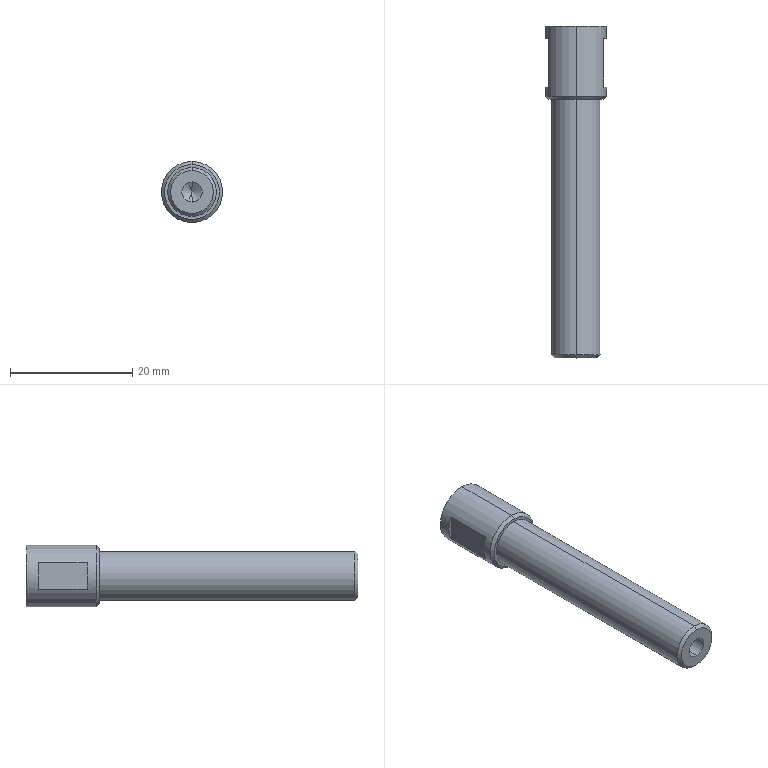Part | SolidWorks | features 3DProfileFeature 2, HoleWzd 2, ICE 2, Chamfer 1, Extrusion 1 | 1 solid | 25 faces | box 10 x 54.3 x 10 mm | volume 2772 mm3 | plane 9 | cone 8 | cylinder 8 | commonest cylinder face diameters 3.3 x2 4.2 x2 8 x2 10 x2
STEP:
#1=CARTESIAN_POINT('',(0.,0.,-3.5));
#2=VERTEX_POINT('',#1);
#3=CARTESIAN_POINT('',(0.,0.,3.5));
#4=VERTEX_POINT('',#3);
#5=CARTESIAN_POINT('',(0.,0.,0.));
#6=DIRECTION('',(0.,-1.,0.));
#7=DIRECTION('',(0.,0.,1.));
#8=AXIS2_PLACEMENT_3D('',#5,#6,#7);
#9=CIRCLE('',#8,3.5);
#10=EDGE_CURVE('',#2,#4,#9,.T.);
#11=ORIENTED_EDGE('',*,*,#10,.F.);
#12=CARTESIAN_POINT('',(0.,0.5,-4.));
#13=VERTEX_POINT('',#12);
#14=CARTESIAN_POINT('',(0.,0.5,-4.));
#15=DIRECTION('',(0.,0.7071,-0.7071));
#16=VECTOR('',#15,1000.);
#17=LINE('',#14,#16);
#18=EDGE_CURVE('',#2,#13,#17,.T.);
#19=ORIENTED_EDGE('',*,*,#18,.T.);
#20=CARTESIAN_POINT('',(0.,0.5,4.));
#21=VERTEX_POINT('',#20);
#22=CARTESIAN_POINT('',(0.,0.5,0.));
#23=DIRECTION('',(0.,1.,0.));
#24=DIRECTION('',(0.,0.,1.));
#25=AXIS2_PLACEMENT_3D('',#22,#23,#24);
#26=CIRCLE('',#25,4.);
#27=EDGE_CURVE('',#21,#13,#26,.T.);
#28=ORIENTED_EDGE('',*,*,#27,.F.);
#29=CARTESIAN_POINT('',(0.,0.5,4.));
#30=DIRECTION('',(0.,0.7071,0.7071));
#31=VECTOR('',#30,1000.);
#32=LINE('',#29,#31);
#33=EDGE_CURVE('',#4,#21,#32,.T.);
#34=ORIENTED_EDGE('',*,*,#33,.F.);
#35=EDGE_LOOP('',(#11,#19,#28,#34));
#36=FACE_OUTER_BOUND('',#35,.T.);
#37=CARTESIAN_POINT('',(0.,0.5,0.));
#38=DIRECTION('',(0.,1.,0.));
#39=DIRECTION('',(0.,0.,1.));
#40=AXIS2_PLACEMENT_3D('',#37,#38,#39);
#41=CONICAL_SURFACE('',#40,4.,0.7854);
#42=ADVANCED_FACE('',(#36),#41,.T.);
#43=CARTESIAN_POINT('',(0.,42.3,-4.5));
#44=VERTEX_POINT('',#43);
#45=CARTESIAN_POINT('',(0.,42.3,4.5));
#46=VERTEX_POINT('',#45);
#47=CARTESIAN_POINT('',(0.,42.3,0.));
#48=DIRECTION('',(0.,-1.,0.));
#49=DIRECTION('',(0.,0.,1.));
#50=AXIS2_PLACEMENT_3D('',#47,#48,#49);
#51=CIRCLE('',#50,4.5);
#52=EDGE_CURVE('',#44,#46,#51,.T.);
#53=ORIENTED_EDGE('',*,*,#52,.F.);
#54=CARTESIAN_POINT('',(0.,42.8,-5.));
#55=VERTEX_POINT('',#54);
#56=CARTESIAN_POINT('',(0.,42.8,-5.));
#57=DIRECTION('',(0.,0.7071,-0.7071));
#58=VECTOR('',#57,1000.);
#59=LINE('',#56,#58);
#60=EDGE_CURVE('',#44,#55,#59,.T.);
#61=ORIENTED_EDGE('',*,*,#60,.T.);
#62=CARTESIAN_POINT('',(0.,42.8,5.));
#63=VERTEX_POINT('',#62);
#64=CARTESIAN_POINT('',(0.,42.8,0.));
#65=DIRECTION('',(0.,1.,0.));
#66=DIRECTION('',(0.,0.,1.));
#67=AXIS2_PLACEMENT_3D('',#64,#65,#66);
#68=CIRCLE('',#67,5.);
#69=EDGE_CURVE('',#63,#55,#68,.T.);
#70=ORIENTED_EDGE('',*,*,#69,.F.);
#71=CARTESIAN_POINT('',(0.,42.8,5.));
#72=DIRECTION('',(0.,0.7071,0.7071));
#73=VECTOR('',#72,1000.);
#74=LINE('',#71,#73);
#75=EDGE_CURVE('',#46,#63,#74,.T.);
#76=ORIENTED_EDGE('',*,*,#75,.F.);
#77=EDGE_LOOP('',(#53,#61,#70,#76));
#78=FACE_OUTER_BOUND('',#77,.T.);
#79=CARTESIAN_POINT('',(0.,42.8,0.));
#80=DIRECTION('',(0.,1.,0.));
#81=DIRECTION('',(0.,0.,1.));
#82=AXIS2_PLACEMENT_3D('',#79,#80,#81);
#83=CONICAL_SURFACE('',#82,5.,0.7854);
#84=ADVANCED_FACE('',(#78),#83,.T.);
#85=CARTESIAN_POINT('',(0.,10.1,1.65));
#86=VERTEX_POINT('',#85);
#87=CARTESIAN_POINT('',(0.,10.1,-1.65));
#88=VERTEX_POINT('',#87);
#89=CARTESIAN_POINT('',(0.,10.1,0.));
#90=DIRECTION('',(0.,-1.,0.));
#91=DIRECTION('',(0.,0.,-1.));
#92=AXIS2_PLACEMENT_3D('',#89,#90,#91);
#93=CIRCLE('',#92,1.65);
#94=EDGE_CURVE('',#86,#88,#93,.T.);
#95=ORIENTED_EDGE('',*,*,#94,.F.);
#96=CARTESIAN_POINT('',(0.,0.,1.65));
#97=VERTEX_POINT('',#96);
#98=CARTESIAN_POINT('',(0.,0.,1.65));
#99=DIRECTION('',(0.,-1.,0.));
#100=VECTOR('',#99,1000.);
#101=LINE('',#98,#100);
#102=EDGE_CURVE('',#86,#97,#101,.T.);
#103=ORIENTED_EDGE('',*,*,#102,.T.);
#104=CARTESIAN_POINT('',(0.,0.,-1.65));
#105=VERTEX_POINT('',#104);
#106=CARTESIAN_POINT('',(0.,0.,0.));
#107=DIRECTION('',(0.,-1.,0.));
#108=DIRECTION('',(0.,0.,-1.));
#109=AXIS2_PLACEMENT_3D('',#106,#107,#108);
#110=CIRCLE('',#109,1.65);
#111=EDGE_CURVE('',#97,#105,#110,.T.);
#112=ORIENTED_EDGE('',*,*,#111,.T.);
#113=CARTESIAN_POINT('',(0.,0.,-1.65));
#114=DIRECTION('',(0.,-1.,0.));
#115=VECTOR('',#114,1000.);
#116=LINE('',#113,#115);
#117=EDGE_CURVE('',#88,#105,#116,.T.);
#118=ORIENTED_EDGE('',*,*,#117,.F.);
#119=EDGE_LOOP('',(#95,#103,#112,#118));
#120=FACE_OUTER_BOUND('',#119,.T.);
#121=CARTESIAN_POINT('',(0.,0.,0.));
#122=DIRECTION('',(0.,-1.,0.));
#123=DIRECTION('',(0.,0.,-1.));
#124=AXIS2_PLACEMENT_3D('',#121,#122,#123);
#125=CYLINDRICAL_SURFACE('',#124,1.65);
#126=ADVANCED_FACE('',(#120),#125,.F.);
#127=CARTESIAN_POINT('',(0.,11.091,0.));
#128=VERTEX_POINT('',#127);
#129=CARTESIAN_POINT('',(0.,10.1,-1.65));
#130=DIRECTION('',(0.,-0.515,-0.8572));
#131=VECTOR('',#130,1000.);
#132=LINE('',#129,#131);
#133=EDGE_CURVE('',#128,#88,#132,.T.);
#134=ORIENTED_EDGE('',*,*,#133,.F.);
#135=CARTESIAN_POINT('',(0.,10.1,1.65));
#136=DIRECTION('',(0.,-0.515,0.8572));
#137=VECTOR('',#136,1000.);
#138=LINE('',#135,#137);
#139=EDGE_CURVE('',#128,#86,#138,.T.);
#140=ORIENTED_EDGE('',*,*,#139,.T.);
#141=ORIENTED_EDGE('',*,*,#94,.T.);
#142=EDGE_LOOP('',(#134,#140,#141));
#143=FACE_OUTER_BOUND('',#142,.T.);
#144=CARTESIAN_POINT('',(0.,10.1,0.));
#145=DIRECTION('',(0.,-1.,0.));
#146=DIRECTION('',(0.,0.,-1.));
#147=AXIS2_PLACEMENT_3D('',#144,#145,#146);
#148=CONICAL_SURFACE('',#147,1.65,1.03);
#149=ADVANCED_FACE('',(#143),#148,.F.);
#150=CARTESIAN_POINT('',(0.,41.9,-2.1));
#151=VERTEX_POINT('',#150);
#152=CARTESIAN_POINT('',(0.,41.9,2.1));
#153=VERTEX_POINT('',#152);
#154=CARTESIAN_POINT('',(0.,41.9,0.));
#155=DIRECTION('',(0.,1.,0.));
#156=DIRECTION('',(0.,0.,1.));
#157=AXIS2_PLACEMENT_3D('',#154,#155,#156);
#158=CIRCLE('',#157,2.1);
#159=EDGE_CURVE('',#151,#153,#158,.T.);
#160=ORIENTED_EDGE('',*,*,#159,.F.);
#161=CARTESIAN_POINT('',(0.,54.3,-2.1));
#162=VERTEX_POINT('',#161);
#163=CARTESIAN_POINT('',(0.,54.3,-2.1));
#164=DIRECTION('',(0.,1.,0.));
#165=VECTOR('',#164,1000.);
#166=LINE('',#163,#165);
#167=EDGE_CURVE('',#151,#162,#166,.T.);
#168=ORIENTED_EDGE('',*,*,#167,.T.);
#169=CARTESIAN_POINT('',(0.,54.3,2.1));
#170=VERTEX_POINT('',#169);
#171=CARTESIAN_POINT('',(0.,54.3,0.));
#172=DIRECTION('',(0.,1.,0.));
#173=DIRECTION('',(0.,0.,1.));
#174=AXIS2_PLACEMENT_3D('',#171,#172,#173);
#175=CIRCLE('',#174,2.1);
#176=EDGE_CURVE('',#162,#170,#175,.T.);
#177=ORIENTED_EDGE('',*,*,#176,.T.);
#178=CARTESIAN_POINT('',(0.,54.3,2.1));
#179=DIRECTION('',(0.,1.,0.));
#180=VECTOR('',#179,1000.);
#181=LINE('',#178,#180);
#182=EDGE_CURVE('',#153,#170,#181,.T.);
#183=ORIENTED_EDGE('',*,*,#182,.F.);
#184=EDGE_LOOP('',(#160,#168,#177,#183));
#185=FACE_OUTER_BOUND('',#184,.T.);
#186=CARTESIAN_POINT('',(0.,54.3,0.));
#187=DIRECTION('',(0.,1.,0.));
#188=DIRECTION('',(0.,0.,1.));
#189=AXIS2_PLACEMENT_3D('',#186,#187,#188);
#190=CYLINDRICAL_SURFACE('',#189,2.1);
#191=ADVANCED_FACE('',(#185),#190,.F.);
#192=CARTESIAN_POINT('',(0.,40.638,0.));
#193=VERTEX_POINT('',#192);
#194=CARTESIAN_POINT('',(0.,41.9,2.1));
#195=DIRECTION('',(0.,0.515,0.8572));
#196=VECTOR('',#195,1000.);
#197=LINE('',#194,#196);
#198=EDGE_CURVE('',#193,#153,#197,.T.);
#199=ORIENTED_EDGE('',*,*,#198,.F.);
#200=CARTESIAN_POINT('',(0.,41.9,-2.1));
#201=DIRECTION('',(0.,0.515,-0.8572));
#202=VECTOR('',#201,1000.);
#203=LINE('',#200,#202);
#204=EDGE_CURVE('',#193,#151,#203,.T.);
#205=ORIENTED_EDGE('',*,*,#204,.T.);
#206=ORIENTED_EDGE('',*,*,#159,.T.);
#207=EDGE_LOOP('',(#199,#205,#206));
#208=FACE_OUTER_BOUND('',#207,.T.);
#209=CARTESIAN_POINT('',(0.,41.9,0.));
#210=DIRECTION('',(0.,1.,0.));
#211=DIRECTION('',(0.,0.,1.));
#212=AXIS2_PLACEMENT_3D('',#209,#210,#211);
#213=CONICAL_SURFACE('',#212,2.1,1.03);
#214=ADVANCED_FACE('',(#208),#213,.F.);
#215=CARTESIAN_POINT('',(4.5,52.3,-2.179));
#216=VERTEX_POINT('',#215);
#217=CARTESIAN_POINT('',(4.5,44.3,-2.179));
#218=VERTEX_POINT('',#217);
#219=CARTESIAN_POINT('',(4.5,54.3,-2.179));
#220=DIRECTION('',(0.,-1.,0.));
#221=VECTOR('',#220,1000.);
#222=LINE('',#219,#221);
#223=EDGE_CURVE('',#216,#218,#222,.T.);
#224=ORIENTED_EDGE('',*,*,#223,.T.);
#225=CARTESIAN_POINT('',(4.5,44.3,2.179));
#226=VERTEX_POINT('',#225);
#227=CARTESIAN_POINT('',(0.,44.3,0.));
#228=DIRECTION('',(0.,-1.,0.));
#229=DIRECTION('',(0.,0.,-1.));
#230=AXIS2_PLACEMENT_3D('',#227,#228,#229);
#231=CIRCLE('',#230,5.);
#232=EDGE_CURVE('',#218,#226,#231,.T.);
#233=ORIENTED_EDGE('',*,*,#232,.T.);
#234=CARTESIAN_POINT('',(4.5,52.3,2.179));
#235=VERTEX_POINT('',#234);
#236=CARTESIAN_POINT('',(4.5,54.3,2.179));
#237=DIRECTION('',(0.,1.,0.));
#238=VECTOR('',#237,1000.);
#239=LINE('',#236,#238);
#240=EDGE_CURVE('',#226,#235,#239,.T.);
#241=ORIENTED_EDGE('',*,*,#240,.T.);
#242=CARTESIAN_POINT('',(0.,52.3,0.));
#243=DIRECTION('',(0.,1.,0.));
#244=DIRECTION('',(0.,0.,1.));
#245=AXIS2_PLACEMENT_3D('',#242,#243,#244);
#246=CIRCLE('',#245,5.);
#247=EDGE_CURVE('',#235,#216,#246,.T.);
#248=ORIENTED_EDGE('',*,*,#247,.T.);
#249=EDGE_LOOP('',(#224,#233,#241,#248));
#250=FACE_BOUND('',#249,.T.);
#251=CARTESIAN_POINT('',(0.,54.3,5.));
#252=VERTEX_POINT('',#251);
#253=CARTESIAN_POINT('',(0.,54.3,-5.));
#254=VERTEX_POINT('',#253);
#255=CARTESIAN_POINT('',(0.,54.3,0.));
#256=DIRECTION('',(0.,1.,0.));
#257=DIRECTION('',(0.,0.,1.));
#258=AXIS2_PLACEMENT_3D('',#255,#256,#257);
#259=CIRCLE('',#258,5.);
#260=EDGE_CURVE('',#252,#254,#259,.T.);
#261=ORIENTED_EDGE('',*,*,#260,.F.);
#262=CARTESIAN_POINT('',(0.,54.3,5.));
#263=DIRECTION('',(0.,-1.,0.));
#264=VECTOR('',#263,1000.);
#265=LINE('',#262,#264);
#266=EDGE_CURVE('',#252,#63,#265,.T.);
#267=ORIENTED_EDGE('',*,*,#266,.T.);
#268=ORIENTED_EDGE('',*,*,#69,.T.);
#269=CARTESIAN_POINT('',(0.,54.3,-5.));
#270=DIRECTION('',(0.,-1.,0.));
#271=VECTOR('',#270,1000.);
#272=LINE('',#269,#271);
#273=EDGE_CURVE('',#254,#55,#272,.T.);
#274=ORIENTED_EDGE('',*,*,#273,.F.);
#275=EDGE_LOOP('',(#261,#267,#268,#274));
#276=FACE_OUTER_BOUND('',#275,.T.);
#277=CARTESIAN_POINT('',(0.,54.3,0.));
#278=DIRECTION('',(0.,-1.,0.));
#279=DIRECTION('',(0.,0.,-1.));
#280=AXIS2_PLACEMENT_3D('',#277,#278,#279);
#281=CYLINDRICAL_SURFACE('',#280,5.);
#282=ADVANCED_FACE('',(#250,#276),#281,.T.);
#283=CARTESIAN_POINT('',(0.,42.3,4.));
#284=VERTEX_POINT('',#283);
#285=CARTESIAN_POINT('',(0.,42.3,-4.));
#286=VERTEX_POINT('',#285);
#287=CARTESIAN_POINT('',(0.,42.3,0.));
#288=DIRECTION('',(0.,1.,0.));
#289=DIRECTION('',(0.,0.,1.));
#290=AXIS2_PLACEMENT_3D('',#287,#288,#289);
#291=CIRCLE('',#290,4.);
#292=EDGE_CURVE('',#284,#286,#291,.T.);
#293=ORIENTED_EDGE('',*,*,#292,.F.);
#294=CARTESIAN_POINT('',(0.,42.3,4.));
#295=DIRECTION('',(0.,-1.,0.));
#296=VECTOR('',#295,1000.);
#297=LINE('',#294,#296);
#298=EDGE_CURVE('',#284,#21,#297,.T.);
#299=ORIENTED_EDGE('',*,*,#298,.T.);
#300=ORIENTED_EDGE('',*,*,#27,.T.);
#301=CARTESIAN_POINT('',(0.,42.3,-4.));
#302=DIRECTION('',(0.,-1.,0.));
#303=VECTOR('',#302,1000.);
#304=LINE('',#301,#303);
#305=EDGE_CURVE('',#286,#13,#304,.T.);
#306=ORIENTED_EDGE('',*,*,#305,.F.);
#307=EDGE_LOOP('',(#293,#299,#300,#306));
#308=FACE_OUTER_BOUND('',#307,.T.);
#309=CARTESIAN_POINT('',(0.,42.3,0.));
#310=DIRECTION('',(0.,-1.,0.));
#311=DIRECTION('',(0.,0.,-1.));
#312=AXIS2_PLACEMENT_3D('',#309,#310,#311);
#313=CYLINDRICAL_SURFACE('',#312,4.);
#314=ADVANCED_FACE('',(#308),#313,.T.);
#315=ORIENTED_EDGE('',*,*,#298,.F.);
#316=CARTESIAN_POINT('',(0.,42.3,0.));
#317=DIRECTION('',(0.,1.,0.));
#318=DIRECTION('',(0.,0.,1.));
#319=AXIS2_PLACEMENT_3D('',#316,#317,#318);
#320=CIRCLE('',#319,4.);
#321=EDGE_CURVE('',#286,#284,#320,.T.);
#322=ORIENTED_EDGE('',*,*,#321,.F.);
#323=ORIENTED_EDGE('',*,*,#305,.T.);
#324=CARTESIAN_POINT('',(0.,0.5,0.));
#325=DIRECTION('',(0.,1.,0.));
#326=DIRECTION('',(0.,0.,1.));
#327=AXIS2_PLACEMENT_3D('',#324,#325,#326);
#328=CIRCLE('',#327,4.);
#329=EDGE_CURVE('',#13,#21,#328,.T.);
#330=ORIENTED_EDGE('',*,*,#329,.T.);
#331=EDGE_LOOP('',(#315,#322,#323,#330));
#332=FACE_OUTER_BOUND('',#331,.T.);
#333=CARTESIAN_POINT('',(0.,42.3,0.));
#334=DIRECTION('',(0.,-1.,0.));
#335=DIRECTION('',(0.,0.,-1.));
#336=AXIS2_PLACEMENT_3D('',#333,#334,#335);
#337=CYLINDRICAL_SURFACE('',#336,4.);
#338=ADVANCED_FACE('',(#332),#337,.T.);
#339=CARTESIAN_POINT('',(0.,0.,0.));
#340=DIRECTION('',(0.,-1.,0.));
#341=DIRECTION('',(0.,0.,1.));
#342=AXIS2_PLACEMENT_3D('',#339,#340,#341);
#343=CIRCLE('',#342,3.5);
#344=EDGE_CURVE('',#4,#2,#343,.T.);
#345=ORIENTED_EDGE('',*,*,#344,.T.);
#346=ORIENTED_EDGE('',*,*,#10,.T.);
#347=EDGE_LOOP('',(#345,#346));
#348=FACE_OUTER_BOUND('',#347,.T.);
#349=CARTESIAN_POINT('',(0.,0.,0.));
#350=DIRECTION('',(0.,-1.,0.));
#351=DIRECTION('',(0.,0.,-1.));
#352=AXIS2_PLACEMENT_3D('',#349,#350,#351);
#353=CIRCLE('',#352,1.65);
#354=EDGE_CURVE('',#105,#97,#353,.T.);
#355=ORIENTED_EDGE('',*,*,#354,.F.);
#356=ORIENTED_EDGE('',*,*,#111,.F.);
#357=EDGE_LOOP('',(#355,#356));
#358=FACE_BOUND('',#357,.T.);
#359=CARTESIAN_POINT('',(0.,0.,0.));
#360=DIRECTION('',(0.,1.,0.));
#361=DIRECTION('',(0.,0.,1.));
#362=AXIS2_PLACEMENT_3D('',#359,#360,#361);
#363=PLANE('',#362);
#364=ADVANCED_FACE('',(#348,#358),#363,.F.);
#365=CARTESIAN_POINT('',(0.,42.3,0.));
#366=DIRECTION('',(0.,-1.,0.));
#367=DIRECTION('',(0.,0.,1.));
#368=AXIS2_PLACEMENT_3D('',#365,#366,#367);
#369=CIRCLE('',#368,4.5);
#370=EDGE_CURVE('',#46,#44,#369,.T.);
#371=ORIENTED_EDGE('',*,*,#370,.T.);
#372=ORIENTED_EDGE('',*,*,#52,.T.);
#373=EDGE_LOOP('',(#371,#372));
#374=FACE_OUTER_BOUND('',#373,.T.);
#375=ORIENTED_EDGE('',*,*,#321,.T.);
#376=ORIENTED_EDGE('',*,*,#292,.T.);
#377=EDGE_LOOP('',(#375,#376));
#378=FACE_BOUND('',#377,.T.);
#379=CARTESIAN_POINT('',(0.,42.3,0.));
#380=DIRECTION('',(0.,1.,0.));
#381=DIRECTION('',(0.,0.,1.));
#382=AXIS2_PLACEMENT_3D('',#379,#380,#381);
#383=PLANE('',#382);
#384=ADVANCED_FACE('',(#374,#378),#383,.F.);
#385=ORIENTED_EDGE('',*,*,#266,.F.);
#386=CARTESIAN_POINT('',(0.,54.3,0.));
#387=DIRECTION('',(0.,1.,0.));
#388=DIRECTION('',(0.,0.,1.));
#389=AXIS2_PLACEMENT_3D('',#386,#387,#388);
#390=CIRCLE('',#389,5.);
#391=EDGE_CURVE('',#254,#252,#390,.T.);
#392=ORIENTED_EDGE('',*,*,#391,.F.);
#393=ORIENTED_EDGE('',*,*,#273,.T.);
#394=CARTESIAN_POINT('',(0.,42.8,0.));
#395=DIRECTION('',(0.,1.,0.));
#396=DIRECTION('',(0.,0.,1.));
#397=AXIS2_PLACEMENT_3D('',#394,#395,#396);
#398=CIRCLE('',#397,5.);
#399=EDGE_CURVE('',#55,#63,#398,.T.);
#400=ORIENTED_EDGE('',*,*,#399,.T.);
#401=EDGE_LOOP('',(#385,#392,#393,#400));
#402=FACE_OUTER_BOUND('',#401,.T.);
#403=CARTESIAN_POINT('',(-4.5,52.3,2.179));
#404=VERTEX_POINT('',#403);
#405=CARTESIAN_POINT('',(-4.5,44.3,2.179));
#406=VERTEX_POINT('',#405);
#407=CARTESIAN_POINT('',(-4.5,54.3,2.179));
#408=DIRECTION('',(0.,-1.,0.));
#409=VECTOR('',#408,1000.);
#410=LINE('',#407,#409);
#411=EDGE_CURVE('',#404,#406,#410,.T.);
#412=ORIENTED_EDGE('',*,*,#411,.T.);
#413=CARTESIAN_POINT('',(-4.5,44.3,-2.179));
#414=VERTEX_POINT('',#413);
#415=CARTESIAN_POINT('',(0.,44.3,0.));
#416=DIRECTION('',(0.,-1.,0.));
#417=DIRECTION('',(0.,0.,-1.));
#418=AXIS2_PLACEMENT_3D('',#415,#416,#417);
#419=CIRCLE('',#418,5.);
#420=EDGE_CURVE('',#406,#414,#419,.T.);
#421=ORIENTED_EDGE('',*,*,#420,.T.);
#422=CARTESIAN_POINT('',(-4.5,52.3,-2.179));
#423=VERTEX_POINT('',#422);
#424=CARTESIAN_POINT('',(-4.5,54.3,-2.179));
#425=DIRECTION('',(0.,1.,0.));
#426=VECTOR('',#425,1000.);
#427=LINE('',#424,#426);
#428=EDGE_CURVE('',#414,#423,#427,.T.);
#429=ORIENTED_EDGE('',*,*,#428,.T.);
#430=CARTESIAN_POINT('',(0.,52.3,0.));
#431=DIRECTION('',(0.,1.,0.));
#432=DIRECTION('',(0.,0.,1.));
#433=AXIS2_PLACEMENT_3D('',#430,#431,#432);
#434=CIRCLE('',#433,5.);
#435=EDGE_CURVE('',#423,#404,#434,.T.);
#436=ORIENTED_EDGE('',*,*,#435,.T.);
#437=EDGE_LOOP('',(#412,#421,#429,#436));
#438=FACE_BOUND('',#437,.T.);
#439=CARTESIAN_POINT('',(0.,54.3,0.));
#440=DIRECTION('',(0.,-1.,0.));
#441=DIRECTION('',(0.,0.,-1.));
#442=AXIS2_PLACEMENT_3D('',#439,#440,#441);
#443=CYLINDRICAL_SURFACE('',#442,5.);
#444=ADVANCED_FACE('',(#402,#438),#443,.T.);
#445=CARTESIAN_POINT('',(0.,54.3,0.));
#446=DIRECTION('',(0.,1.,0.));
#447=DIRECTION('',(0.,0.,1.));
#448=AXIS2_PLACEMENT_3D('',#445,#446,#447);
#449=CIRCLE('',#448,2.1);
#450=EDGE_CURVE('',#170,#162,#449,.T.);
#451=ORIENTED_EDGE('',*,*,#450,.F.);
#452=ORIENTED_EDGE('',*,*,#176,.F.);
#453=EDGE_LOOP('',(#451,#452));
#454=FACE_BOUND('',#453,.T.);
#455=ORIENTED_EDGE('',*,*,#391,.T.);
#456=ORIENTED_EDGE('',*,*,#260,.T.);
#457=EDGE_LOOP('',(#455,#456));
#458=FACE_OUTER_BOUND('',#457,.T.);
#459=CARTESIAN_POINT('',(0.,54.3,0.));
#460=DIRECTION('',(0.,1.,0.));
#461=DIRECTION('',(0.,0.,1.));
#462=AXIS2_PLACEMENT_3D('',#459,#460,#461);
#463=PLANE('',#462);
#464=ADVANCED_FACE('',(#454,#458),#463,.T.);
#465=ORIENTED_EDGE('',*,*,#204,.F.);
#466=ORIENTED_EDGE('',*,*,#198,.T.);
#467=CARTESIAN_POINT('',(0.,41.9,0.));
#468=DIRECTION('',(0.,1.,0.));
#469=DIRECTION('',(0.,0.,1.));
#470=AXIS2_PLACEMENT_3D('',#467,#468,#469);
#471=CIRCLE('',#470,2.1);
#472=EDGE_CURVE('',#153,#151,#471,.T.);
#473=ORIENTED_EDGE('',*,*,#472,.T.);
#474=EDGE_LOOP('',(#465,#466,#473));
#475=FACE_OUTER_BOUND('',#474,.T.);
#476=CARTESIAN_POINT('',(0.,41.9,0.));
#477=DIRECTION('',(0.,1.,0.));
#478=DIRECTION('',(0.,0.,1.));
#479=AXIS2_PLACEMENT_3D('',#476,#477,#478);
#480=CONICAL_SURFACE('',#479,2.1,1.03);
#481=ADVANCED_FACE('',(#475),#480,.F.);
#482=ORIENTED_EDGE('',*,*,#167,.F.);
#483=ORIENTED_EDGE('',*,*,#472,.F.);
#484=ORIENTED_EDGE('',*,*,#182,.T.);
#485=ORIENTED_EDGE('',*,*,#450,.T.);
#486=EDGE_LOOP('',(#482,#483,#484,#485));
#487=FACE_OUTER_BOUND('',#486,.T.);
#488=CARTESIAN_POINT('',(0.,54.3,0.));
#489=DIRECTION('',(0.,1.,0.));
#490=DIRECTION('',(0.,0.,1.));
#491=AXIS2_PLACEMENT_3D('',#488,#489,#490);
#492=CYLINDRICAL_SURFACE('',#491,2.1);
#493=ADVANCED_FACE('',(#487),#492,.F.);
#494=ORIENTED_EDGE('',*,*,#139,.F.);
#495=ORIENTED_EDGE('',*,*,#133,.T.);
#496=CARTESIAN_POINT('',(0.,10.1,0.));
#497=DIRECTION('',(0.,-1.,0.));
#498=DIRECTION('',(0.,0.,-1.));
#499=AXIS2_PLACEMENT_3D('',#496,#497,#498);
#500=CIRCLE('',#499,1.65);
#501=EDGE_CURVE('',#88,#86,#500,.T.);
#502=ORIENTED_EDGE('',*,*,#501,.T.);
#503=EDGE_LOOP('',(#494,#495,#502));
#504=FACE_OUTER_BOUND('',#503,.T.);
#505=CARTESIAN_POINT('',(0.,10.1,0.));
#506=DIRECTION('',(0.,-1.,0.));
#507=DIRECTION('',(0.,0.,-1.));
#508=AXIS2_PLACEMENT_3D('',#505,#506,#507);
#509=CONICAL_SURFACE('',#508,1.65,1.03);
#510=ADVANCED_FACE('',(#504),#509,.F.);
#511=ORIENTED_EDGE('',*,*,#102,.F.);
#512=ORIENTED_EDGE('',*,*,#501,.F.);
#513=ORIENTED_EDGE('',*,*,#117,.T.);
#514=ORIENTED_EDGE('',*,*,#354,.T.);
#515=EDGE_LOOP('',(#511,#512,#513,#514));
#516=FACE_OUTER_BOUND('',#515,.T.);
#517=CARTESIAN_POINT('',(0.,0.,0.));
#518=DIRECTION('',(0.,-1.,0.));
#519=DIRECTION('',(0.,0.,-1.));
#520=AXIS2_PLACEMENT_3D('',#517,#518,#519);
#521=CYLINDRICAL_SURFACE('',#520,1.65);
#522=ADVANCED_FACE('',(#516),#521,.F.);
#523=CARTESIAN_POINT('',(-4.5,52.3,-5.));
#524=DIRECTION('',(0.,0.,1.));
#525=VECTOR('',#524,1000.);
#526=LINE('',#523,#525);
#527=EDGE_CURVE('',#423,#404,#526,.T.);
#528=ORIENTED_EDGE('',*,*,#527,.F.);
#529=ORIENTED_EDGE('',*,*,#428,.F.);
#530=CARTESIAN_POINT('',(-4.5,44.3,-5.));
#531=DIRECTION('',(0.,0.,1.));
#532=VECTOR('',#531,1000.);
#533=LINE('',#530,#532);
#534=EDGE_CURVE('',#414,#406,#533,.T.);
#535=ORIENTED_EDGE('',*,*,#534,.T.);
#536=ORIENTED_EDGE('',*,*,#411,.F.);
#537=EDGE_LOOP('',(#528,#529,#535,#536));
#538=FACE_OUTER_BOUND('',#537,.T.);
#539=CARTESIAN_POINT('',(-4.5,52.3,-5.));
#540=DIRECTION('',(1.,0.,0.));
#541=DIRECTION('',(0.,0.,-1.));
#542=AXIS2_PLACEMENT_3D('',#539,#540,#541);
#543=PLANE('',#542);
#544=ADVANCED_FACE('',(#538),#543,.F.);
#545=ORIENTED_EDGE('',*,*,#534,.F.);
#546=ORIENTED_EDGE('',*,*,#420,.F.);
#547=EDGE_LOOP('',(#545,#546));
#548=FACE_OUTER_BOUND('',#547,.T.);
#549=CARTESIAN_POINT('',(-5.5,44.3,-5.));
#550=DIRECTION('',(0.,-1.,0.));
#551=DIRECTION('',(0.,0.,-1.));
#552=AXIS2_PLACEMENT_3D('',#549,#550,#551);
#553=PLANE('',#552);
#554=ADVANCED_FACE('',(#548),#553,.F.);
#555=ORIENTED_EDGE('',*,*,#527,.T.);
#556=ORIENTED_EDGE('',*,*,#435,.F.);
#557=EDGE_LOOP('',(#555,#556));
#558=FACE_OUTER_BOUND('',#557,.T.);
#559=CARTESIAN_POINT('',(-5.5,52.3,-5.));
#560=DIRECTION('',(0.,1.,0.));
#561=DIRECTION('',(0.,0.,1.));
#562=AXIS2_PLACEMENT_3D('',#559,#560,#561);
#563=PLANE('',#562);
#564=ADVANCED_FACE('',(#558),#563,.F.);
#565=CARTESIAN_POINT('',(4.5,44.3,-5.));
#566=DIRECTION('',(0.,0.,1.));
#567=VECTOR('',#566,1000.);
#568=LINE('',#565,#567);
#569=EDGE_CURVE('',#218,#226,#568,.T.);
#570=ORIENTED_EDGE('',*,*,#569,.T.);
#571=ORIENTED_EDGE('',*,*,#232,.F.);
#572=EDGE_LOOP('',(#570,#571));
#573=FACE_OUTER_BOUND('',#572,.T.);
#574=CARTESIAN_POINT('',(5.5,44.3,-5.));
#575=DIRECTION('',(0.,-1.,0.));
#576=DIRECTION('',(0.,0.,-1.));
#577=AXIS2_PLACEMENT_3D('',#574,#575,#576);
#578=PLANE('',#577);
#579=ADVANCED_FACE('',(#573),#578,.F.);
#580=CARTESIAN_POINT('',(4.5,52.3,-5.));
#581=DIRECTION('',(0.,0.,1.));
#582=VECTOR('',#581,1000.);
#583=LINE('',#580,#582);
#584=EDGE_CURVE('',#216,#235,#583,.T.);
#585=ORIENTED_EDGE('',*,*,#584,.T.);
#586=ORIENTED_EDGE('',*,*,#240,.F.);
#587=ORIENTED_EDGE('',*,*,#569,.F.);
#588=ORIENTED_EDGE('',*,*,#223,.F.);
#589=EDGE_LOOP('',(#585,#586,#587,#588));
#590=FACE_OUTER_BOUND('',#589,.T.);
#591=CARTESIAN_POINT('',(4.5,52.3,-5.));
#592=DIRECTION('',(-1.,0.,0.));
#593=DIRECTION('',(0.,0.,1.));
#594=AXIS2_PLACEMENT_3D('',#591,#592,#593);
#595=PLANE('',#594);
#596=ADVANCED_FACE('',(#590),#595,.F.);
#597=ORIENTED_EDGE('',*,*,#584,.F.);
#598=ORIENTED_EDGE('',*,*,#247,.F.);
#599=EDGE_LOOP('',(#597,#598));
#600=FACE_OUTER_BOUND('',#599,.T.);
#601=CARTESIAN_POINT('',(5.5,52.3,-5.));
#602=DIRECTION('',(0.,1.,0.));
#603=DIRECTION('',(0.,0.,1.));
#604=AXIS2_PLACEMENT_3D('',#601,#602,#603);
#605=PLANE('',#604);
#606=ADVANCED_FACE('',(#600),#605,.F.);
#607=ORIENTED_EDGE('',*,*,#60,.F.);
#608=ORIENTED_EDGE('',*,*,#370,.F.);
#609=ORIENTED_EDGE('',*,*,#75,.T.);
#610=ORIENTED_EDGE('',*,*,#399,.F.);
#611=EDGE_LOOP('',(#607,#608,#609,#610));
#612=FACE_OUTER_BOUND('',#611,.T.);
#613=CARTESIAN_POINT('',(0.,42.8,0.));
#614=DIRECTION('',(0.,1.,0.));
#615=DIRECTION('',(0.,0.,1.));
#616=AXIS2_PLACEMENT_3D('',#613,#614,#615);
#617=CONICAL_SURFACE('',#616,5.,0.7854);
#618=ADVANCED_FACE('',(#612),#617,.T.);
#619=ORIENTED_EDGE('',*,*,#18,.F.);
#620=ORIENTED_EDGE('',*,*,#344,.F.);
#621=ORIENTED_EDGE('',*,*,#33,.T.);
#622=ORIENTED_EDGE('',*,*,#329,.F.);
#623=EDGE_LOOP('',(#619,#620,#621,#622));
#624=FACE_OUTER_BOUND('',#623,.T.);
#625=CARTESIAN_POINT('',(0.,0.5,0.));
#626=DIRECTION('',(0.,1.,0.));
#627=DIRECTION('',(0.,0.,1.));
#628=AXIS2_PLACEMENT_3D('',#625,#626,#627);
#629=CONICAL_SURFACE('',#628,4.,0.7854);
#630=ADVANCED_FACE('',(#624),#629,.T.);
#631=CLOSED_SHELL('',(#42,#84,#126,#149,#191,#214,#282,#314,#338,#364,#384,#444,#464,#481,#493,#510,#522,#544,#554,#564,#579,#596,#606,#618,#630));
#632=MANIFOLD_SOLID_BREP('',#631);
#633=CARTESIAN_POINT('',(0.,0.,0.));
#634=DIRECTION('',(0.,0.,1.));
#635=DIRECTION('',(1.,0.,0.));
#636=AXIS2_PLACEMENT_3D('',#633,#634,#635);
#637=(LENGTH_UNIT()NAMED_UNIT(*)SI_UNIT(.MILLI.,.METRE.));
#638=UNCERTAINTY_MEASURE_WITH_UNIT(LENGTH_MEASURE(0.00001),#637,'','');
#639=(NAMED_UNIT(*)PLANE_ANGLE_UNIT()SI_UNIT($,.RADIAN.));
#640=(NAMED_UNIT(*)SI_UNIT($,.STERADIAN.)SOLID_ANGLE_UNIT());
#641=(GEOMETRIC_REPRESENTATION_CONTEXT(3)GLOBAL_UNCERTAINTY_ASSIGNED_CONTEXT((#638))GLOBAL_UNIT_ASSIGNED_CONTEXT((#637,#639,#640))REPRESENTATION_CONTEXT('',''));
#642=ADVANCED_BREP_SHAPE_REPRESENTATION('',(#632,#636),#641);